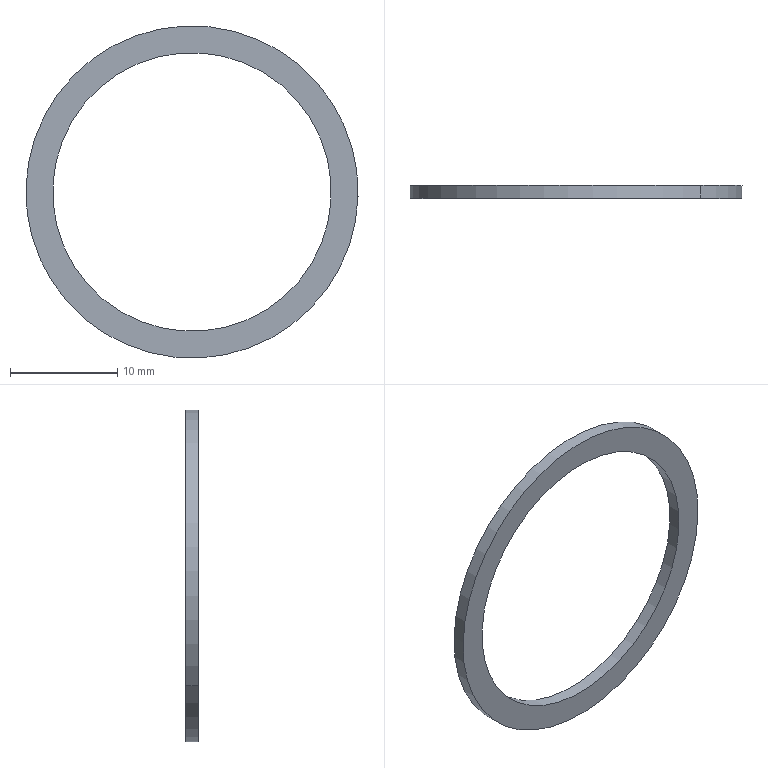Part | STEP file | MSBR-27 | 1 solid | 6 faces | box 31 x 1.2 x 31 mm | volume 268.606 mm3 | cylinder 4 | plane 2 | commonest cylinder face diameters 26 x2 31 x2
STEP:
#1=CARTESIAN_POINT('',(0.,0.,0.));
#2=DIRECTION('',(0.,0.,1.));
#3=DIRECTION('',(1.,0.,0.));
#4=AXIS2_PLACEMENT_3D('',#1,#2,#3);
#5=CARTESIAN_POINT('',(-11.652,-94.03,-10.121));
#6=VERTEX_POINT('',#5);
#7=CARTESIAN_POINT('',(11.652,-94.03,10.321));
#8=VERTEX_POINT('',#7);
#9=CARTESIAN_POINT('',(0.,-94.03,0.1));
#10=DIRECTION('',(0.,-1.,0.));
#11=DIRECTION('',(-0.7518,0.,-0.6594));
#12=AXIS2_PLACEMENT_3D('',#9,#10,#11);
#13=CIRCLE('',#12,15.5);
#14=EDGE_CURVE('',#6,#8,#13,.T.);
#15=ORIENTED_EDGE('',*,*,#14,.T.);
#16=CARTESIAN_POINT('',(0.,-94.03,0.1));
#17=DIRECTION('',(0.,-1.,0.));
#18=DIRECTION('',(0.7518,0.,0.6594));
#19=AXIS2_PLACEMENT_3D('',#16,#17,#18);
#20=CIRCLE('',#19,15.5);
#21=EDGE_CURVE('',#8,#6,#20,.T.);
#22=ORIENTED_EDGE('',*,*,#21,.T.);
#23=EDGE_LOOP('',(#15,#22));
#24=FACE_OUTER_BOUND('',#23,.F.);
#25=CARTESIAN_POINT('',(9.773,-94.03,8.673));
#26=VERTEX_POINT('',#25);
#27=CARTESIAN_POINT('',(-9.773,-94.03,-8.473));
#28=VERTEX_POINT('',#27);
#29=CARTESIAN_POINT('',(0.,-94.03,0.1));
#30=DIRECTION('',(0.,1.,0.));
#31=DIRECTION('',(0.7518,0.,0.6594));
#32=AXIS2_PLACEMENT_3D('',#29,#30,#31);
#33=CIRCLE('',#32,13.);
#34=EDGE_CURVE('',#26,#28,#33,.T.);
#35=ORIENTED_EDGE('',*,*,#34,.T.);
#36=CARTESIAN_POINT('',(0.,-94.03,0.1));
#37=DIRECTION('',(0.,1.,0.));
#38=DIRECTION('',(-0.7518,0.,-0.6594));
#39=AXIS2_PLACEMENT_3D('',#36,#37,#38);
#40=CIRCLE('',#39,13.);
#41=EDGE_CURVE('',#28,#26,#40,.T.);
#42=ORIENTED_EDGE('',*,*,#41,.T.);
#43=EDGE_LOOP('',(#35,#42));
#44=FACE_BOUND('',#43,.F.);
#45=CARTESIAN_POINT('',(0.,-94.03,0.1));
#46=DIRECTION('',(0.,1.,0.));
#47=DIRECTION('',(-0.7518,0.,-0.6594));
#48=AXIS2_PLACEMENT_3D('',#45,#46,#47);
#49=PLANE('',#48);
#50=ADVANCED_FACE('',(#24,#44),#49,.T.);
#51=CARTESIAN_POINT('',(-11.652,-95.23,-10.121));
#52=VERTEX_POINT('',#51);
#53=CARTESIAN_POINT('',(-11.652,-95.23,-10.121));
#54=DIRECTION('',(0.,1.,0.));
#55=VECTOR('',#54,1.2);
#56=LINE('',#53,#55);
#57=EDGE_CURVE('',#52,#6,#56,.T.);
#58=ORIENTED_EDGE('',*,*,#57,.F.);
#59=CARTESIAN_POINT('',(11.652,-95.23,10.321));
#60=VERTEX_POINT('',#59);
#61=CARTESIAN_POINT('',(0.,-95.23,0.1));
#62=DIRECTION('',(0.,1.,0.));
#63=DIRECTION('',(0.7518,0.,0.6594));
#64=AXIS2_PLACEMENT_3D('',#61,#62,#63);
#65=CIRCLE('',#64,15.5);
#66=EDGE_CURVE('',#60,#52,#65,.T.);
#67=ORIENTED_EDGE('',*,*,#66,.F.);
#68=CARTESIAN_POINT('',(11.652,-94.03,10.321));
#69=DIRECTION('',(0.,-1.,0.));
#70=VECTOR('',#69,1.2);
#71=LINE('',#68,#70);
#72=EDGE_CURVE('',#8,#60,#71,.T.);
#73=ORIENTED_EDGE('',*,*,#72,.F.);
#74=ORIENTED_EDGE('',*,*,#14,.F.);
#75=EDGE_LOOP('',(#58,#67,#73,#74));
#76=FACE_OUTER_BOUND('',#75,.F.);
#77=CARTESIAN_POINT('',(0.,-95.304,0.1));
#78=DIRECTION('',(0.,1.,0.));
#79=DIRECTION('',(0.7518,0.,0.6594));
#80=AXIS2_PLACEMENT_3D('',#77,#78,#79);
#81=CYLINDRICAL_SURFACE('',#80,15.5);
#82=ADVANCED_FACE('',(#76),#81,.T.);
#83=CARTESIAN_POINT('',(0.,-95.23,0.1));
#84=DIRECTION('',(0.,1.,0.));
#85=DIRECTION('',(-0.7518,0.,-0.6594));
#86=AXIS2_PLACEMENT_3D('',#83,#84,#85);
#87=CIRCLE('',#86,15.5);
#88=EDGE_CURVE('',#52,#60,#87,.T.);
#89=ORIENTED_EDGE('',*,*,#88,.F.);
#90=ORIENTED_EDGE('',*,*,#57,.T.);
#91=ORIENTED_EDGE('',*,*,#21,.F.);
#92=ORIENTED_EDGE('',*,*,#72,.T.);
#93=EDGE_LOOP('',(#89,#90,#91,#92));
#94=FACE_OUTER_BOUND('',#93,.F.);
#95=CARTESIAN_POINT('',(0.,-95.304,0.1));
#96=DIRECTION('',(0.,1.,0.));
#97=DIRECTION('',(0.7518,0.,0.6594));
#98=AXIS2_PLACEMENT_3D('',#95,#96,#97);
#99=CYLINDRICAL_SURFACE('',#98,15.5);
#100=ADVANCED_FACE('',(#94),#99,.T.);
#101=ORIENTED_EDGE('',*,*,#66,.T.);
#102=ORIENTED_EDGE('',*,*,#88,.T.);
#103=EDGE_LOOP('',(#101,#102));
#104=FACE_OUTER_BOUND('',#103,.F.);
#105=CARTESIAN_POINT('',(-9.773,-95.23,-8.473));
#106=VERTEX_POINT('',#105);
#107=CARTESIAN_POINT('',(9.773,-95.23,8.673));
#108=VERTEX_POINT('',#107);
#109=CARTESIAN_POINT('',(0.,-95.23,0.1));
#110=DIRECTION('',(0.,-1.,0.));
#111=DIRECTION('',(-0.7518,0.,-0.6594));
#112=AXIS2_PLACEMENT_3D('',#109,#110,#111);
#113=CIRCLE('',#112,13.);
#114=EDGE_CURVE('',#106,#108,#113,.T.);
#115=ORIENTED_EDGE('',*,*,#114,.T.);
#116=CARTESIAN_POINT('',(0.,-95.23,0.1));
#117=DIRECTION('',(0.,-1.,0.));
#118=DIRECTION('',(0.7518,0.,0.6594));
#119=AXIS2_PLACEMENT_3D('',#116,#117,#118);
#120=CIRCLE('',#119,13.);
#121=EDGE_CURVE('',#108,#106,#120,.T.);
#122=ORIENTED_EDGE('',*,*,#121,.T.);
#123=EDGE_LOOP('',(#115,#122));
#124=FACE_BOUND('',#123,.F.);
#125=CARTESIAN_POINT('',(0.,-95.23,0.1));
#126=DIRECTION('',(0.,1.,0.));
#127=DIRECTION('',(-0.7518,0.,-0.6594));
#128=AXIS2_PLACEMENT_3D('',#125,#126,#127);
#129=PLANE('',#128);
#130=ADVANCED_FACE('',(#104,#124),#129,.F.);
#131=ORIENTED_EDGE('',*,*,#114,.F.);
#132=CARTESIAN_POINT('',(-9.773,-94.03,-8.473));
#133=DIRECTION('',(0.,-1.,0.));
#134=VECTOR('',#133,1.2);
#135=LINE('',#132,#134);
#136=EDGE_CURVE('',#28,#106,#135,.T.);
#137=ORIENTED_EDGE('',*,*,#136,.F.);
#138=ORIENTED_EDGE('',*,*,#34,.F.);
#139=CARTESIAN_POINT('',(9.773,-95.23,8.673));
#140=DIRECTION('',(0.,1.,0.));
#141=VECTOR('',#140,1.2);
#142=LINE('',#139,#141);
#143=EDGE_CURVE('',#108,#26,#142,.T.);
#144=ORIENTED_EDGE('',*,*,#143,.F.);
#145=EDGE_LOOP('',(#131,#137,#138,#144));
#146=FACE_OUTER_BOUND('',#145,.F.);
#147=CARTESIAN_POINT('',(0.,-95.304,0.1));
#148=DIRECTION('',(0.,1.,0.));
#149=DIRECTION('',(0.7518,0.,0.6594));
#150=AXIS2_PLACEMENT_3D('',#147,#148,#149);
#151=CYLINDRICAL_SURFACE('',#150,13.);
#152=ADVANCED_FACE('',(#146),#151,.F.);
#153=ORIENTED_EDGE('',*,*,#136,.T.);
#154=ORIENTED_EDGE('',*,*,#121,.F.);
#155=ORIENTED_EDGE('',*,*,#143,.T.);
#156=ORIENTED_EDGE('',*,*,#41,.F.);
#157=EDGE_LOOP('',(#153,#154,#155,#156));
#158=FACE_OUTER_BOUND('',#157,.F.);
#159=CARTESIAN_POINT('',(0.,-95.304,0.1));
#160=DIRECTION('',(0.,1.,0.));
#161=DIRECTION('',(0.7518,0.,0.6594));
#162=AXIS2_PLACEMENT_3D('',#159,#160,#161);
#163=CYLINDRICAL_SURFACE('',#162,13.);
#164=ADVANCED_FACE('',(#158),#163,.F.);
#165=CLOSED_SHELL('',(#50,#82,#100,#130,#152,#164));
#166=MANIFOLD_SOLID_BREP('',#165);
#167=(LENGTH_UNIT()NAMED_UNIT(*)SI_UNIT(.MILLI.,.METRE.));
#168=UNCERTAINTY_MEASURE_WITH_UNIT(LENGTH_MEASURE(0.006189),#167,'','');
#169=(NAMED_UNIT(*)PLANE_ANGLE_UNIT()SI_UNIT($,.RADIAN.));
#170=PLANE_ANGLE_MEASURE_WITH_UNIT(PLANE_ANGLE_MEASURE(0.01745),#169);
#171=(CONVERSION_BASED_UNIT('DEGREE',#170)NAMED_UNIT(*)PLANE_ANGLE_UNIT());
#172=(NAMED_UNIT(*)SI_UNIT($,.STERADIAN.)SOLID_ANGLE_UNIT());
#173=(GEOMETRIC_REPRESENTATION_CONTEXT(3)GLOBAL_UNCERTAINTY_ASSIGNED_CONTEXT((#168))GLOBAL_UNIT_ASSIGNED_CONTEXT((#167,#171,#172))REPRESENTATION_CONTEXT('',''));
#174=ADVANCED_BREP_SHAPE_REPRESENTATION('',(#4,#166),#173);